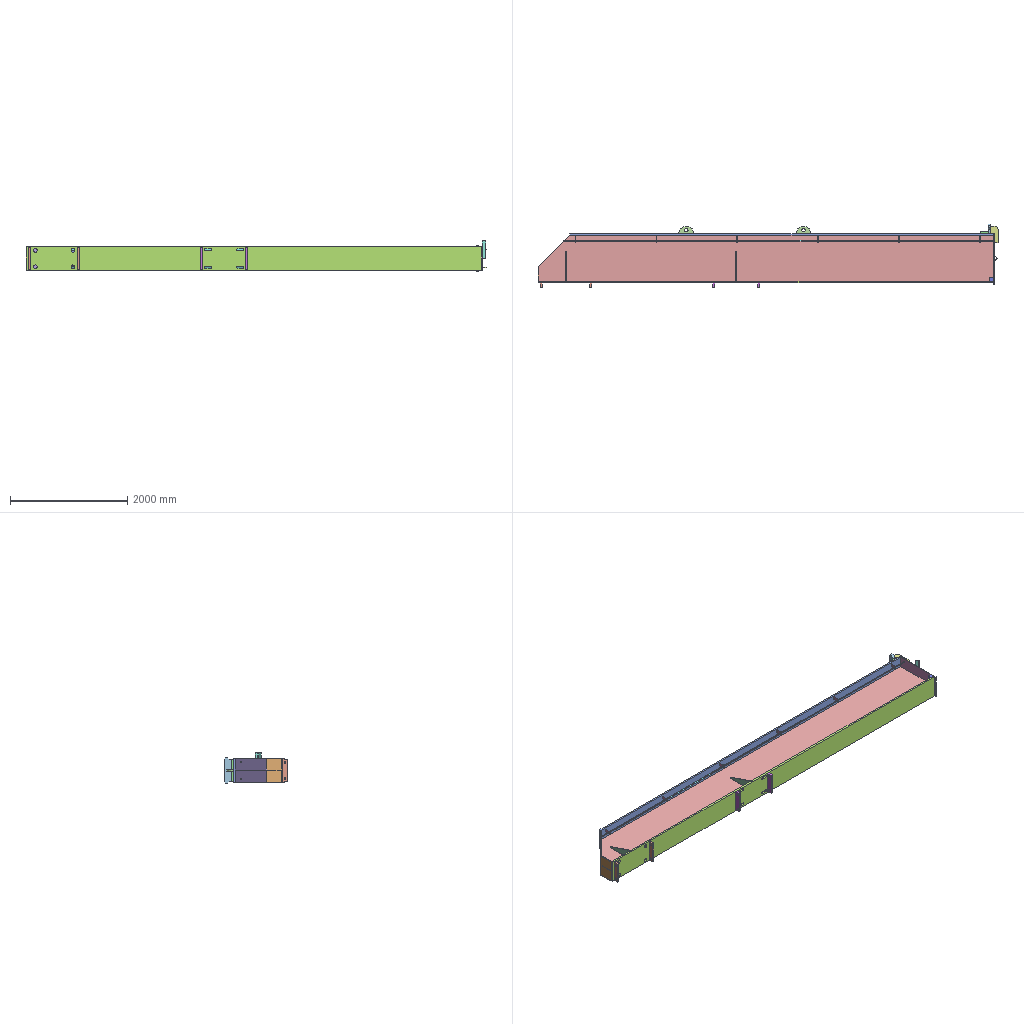Assembly | SolidWorks | 18 different items | 38 placed | box 7846 x 1080 x 514 mm
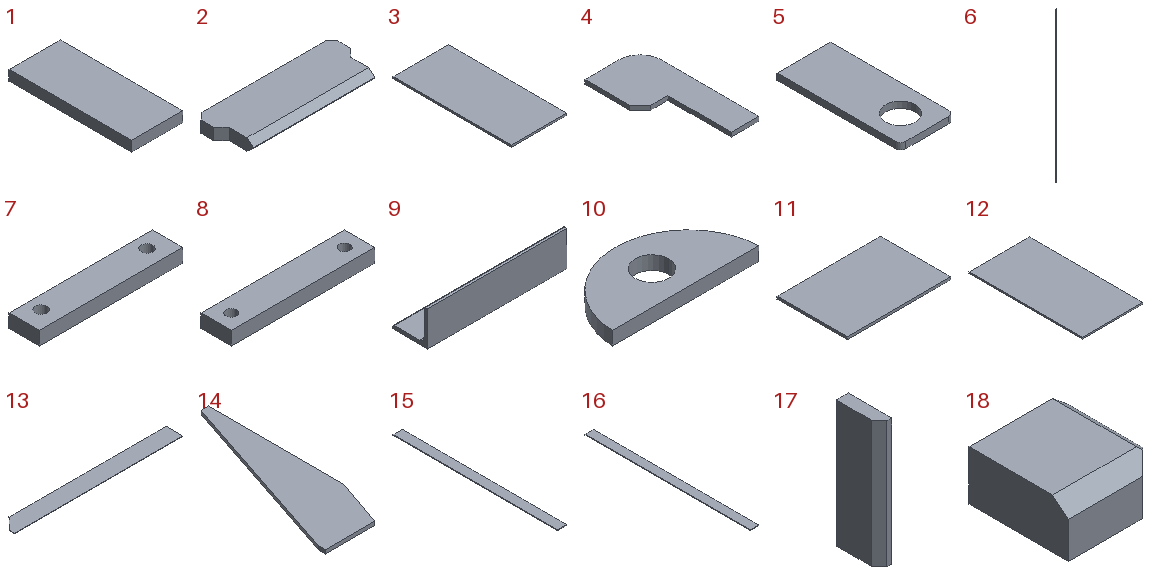Parts list (item | quantity | size | volume | features):
1 | x1 | 50 x 120 x 10 mm | 60000 mm3 | features Extrusion 1
2 | x1 | 428 x 160 x 36 mm | 2167938 mm3 | features Extrusion 1, ICE 1
3 | x1 | 400 x 855 x 14 mm | 4788000 mm3 | features Extrusion 1
4 | x2 | 130 x 280 x 10 mm | 258010 mm3 | features Extrusion 1
5 | x12 | 50 x 115 x 6 mm | 30741 mm3 | features Extrusion 1
6 | x2 | 19.05 x 19.05 x 7329 mm | 1032084 mm3 | features Extrusion 1
7 | x2 | 380 x 80 x 36 mm | 1040206 mm3 | features Extrusion 1, HoleWzd 1
8 | x2 | 380 x 80 x 36 mm | 1049498 mm3 | features Extrusion 1, HoleWzd 1
9 | x1 | 300 x 75 x 75 mm | 345099 mm3 | features Extrusion 1
10 | x2 | 259.808 x 125 x 24 mm | 538064 mm3 | features Extrusion 1
11 | x1 | 400 x 270 x 10 mm | 1080000 mm3 | features Extrusion 1
12 | x1 | 400 x 749 x 10 mm | 2996000 mm3 | features Extrusion 1
13 | x1 | 7756 x 780 x 16 mm | 94547680 mm3 | features Extrusion 1
14 | x4 | 180 x 500 x 10 mm | 486750 mm3 | features Extrusion 1
15 | x1 | 400 x 7226 x 30 mm | 86712000 mm3 | features Extrusion 1
16 | x1 | 400 x 7756 x 30 mm | 93072000 mm3 | features Extrusion 1
17 | x1 | 36 x 130 x 380 mm | 1678543 mm3 | features Extrusion 1
18 | x2 | 60 x 60 x 30 mm | 100955 mm3 | features Chamfer 3, Extrusion 1
Mates (type | each side: item.copy, entity, surface, feature):
Coincident | 13.1 plane | assembly plane | 2 times
DistanceDim | 13.1 plane | assembly plane
Coincident | 15.1 plane | assembly plane
Coincident | 13.1 face plane Boss-Extrude1 | 15.1 face plane Boss-Extrude1 | 2 times
Coincident | 16.1 plane | assembly plane
Coincident | 13.1 face plane Boss-Extrude1 | 16.1 face plane | 2 times
Coincident | 3.1 plane | assembly plane
DistanceDim | 3.1 face plane Boss-Extrude1 | 15.1 face plane Boss-Extrude1
Coincident | 13.1 face plane Boss-Extrude1 | 3.1 face plane Boss-Extrude1
Coincident | 9.1 plane | assembly plane
Tangent | 3.1 face plane Boss-Extrude1 | 9.1 face cylinder Base | 2 times
DistanceDim | 9.1 edge | 15.1 face plane Boss-Extrude1
Coincident | 11.1 plane | assembly plane
Coincident | 13.1 face plane Boss-Extrude1 | 11.1 face plane Boss-Extrude1
DistanceDim | 11.1 face plane Boss-Extrude1 | 16.1 face plane
Coincident | 12.1 plane | assembly plane
Coincident | 13.1 face plane Boss-Extrude1 | 12.1 face plane Boss-Extrude1
Coincident | 11.1 face plane Boss-Extrude1 | 12.1 edge
DistanceDim | 4.1 face plane Boss-Extrude1 | assembly plane
Coincident | 15.1 face plane Boss-Extrude1 | 4.1 face plane Boss-Extrude1
Coincident | 2.1 plane | assembly plane
Coincident | 15.1 face plane Boss-Extrude1 | 2.1 face plane Boss-Extrude1
DistanceDim | 2.1 face plane Boss-Extrude1 | 3.1 face plane Boss-Extrude1
Coincident | 2.1 face plane Boss-Extrude1 | 4.1 face plane Boss-Extrude1
Coincident | 17.1 plane | assembly plane
Coincident | 15.1 face plane Boss-Extrude1 | 17.1 face plane Boss-Extrude1
Coincident | 17.1 face plane Boss-Extrude1 | 2.1 face plane Boss-Extrude1
Coincident | 1.1 plane | assembly plane
Coincident | 17.1 face plane Boss-Extrude1 | 1.1 face plane Boss-Extrude1
Coincident | 1.1 face plane Boss-Extrude1 | 2.1 face plane Boss-Extrude1
DistanceDim | 14.1 plane | 3.1 face plane Boss-Extrude1
Coincident | 13.1 face plane Boss-Extrude1 | 14.1 face plane Boss-Extrude1
Coincident | 16.1 face plane | 14.1 face plane Boss-Extrude1
Coincident | 16.1 face plane | 8.1 face plane Boss-Extrude1
DistanceDim | 14.1 plane | 8.1 face plane Boss-Extrude1
Coincident | 8.1 plane | assembly plane
Coincident | 7.1 plane | assembly plane
Coincident | 16.1 face plane | 7.1 face plane Boss-Extrude1
DistanceDim | 14.2 plane | 7.1 face plane Boss-Extrude1
Coincident | 18.1 face plane Boss-Extrude1 | 16.1 face plane
Coincident | 3.1 face plane Boss-Extrude1 | 18.1 face plane Boss-Extrude1
Coincident | 16.1 face plane | 18.1 face plane Boss-Extrude1
Coincident | 16.1 face plane | 18.2 face plane Boss-Extrude1 | 2 times
Coincident | 3.1 face plane Boss-Extrude1 | 18.2 face plane Boss-Extrude1
Coincident | 15.1 face plane Boss-Extrude1 | 10.1 face plane Boss-Extrude1
Coincident | 10.1 plane | assembly plane
DistanceDim | 10.1 plane | assembly plane
Coincident | 15.1 face plane Boss-Extrude1 | 5.1 face plane Boss-Extrude1
DistanceDim | 5.1 plane | 15.1 face plane Boss-Extrude1
DistanceDim | 5.1 plane | 3.1 face plane Boss-Extrude1
Concentric | 5.1 face cylinder Boss-Extrude1 | 6.1 face cylinder Boss-Extrude1
Coincident | 3.1 face plane Boss-Extrude1 | 6.1 face plane Boss-Extrude1